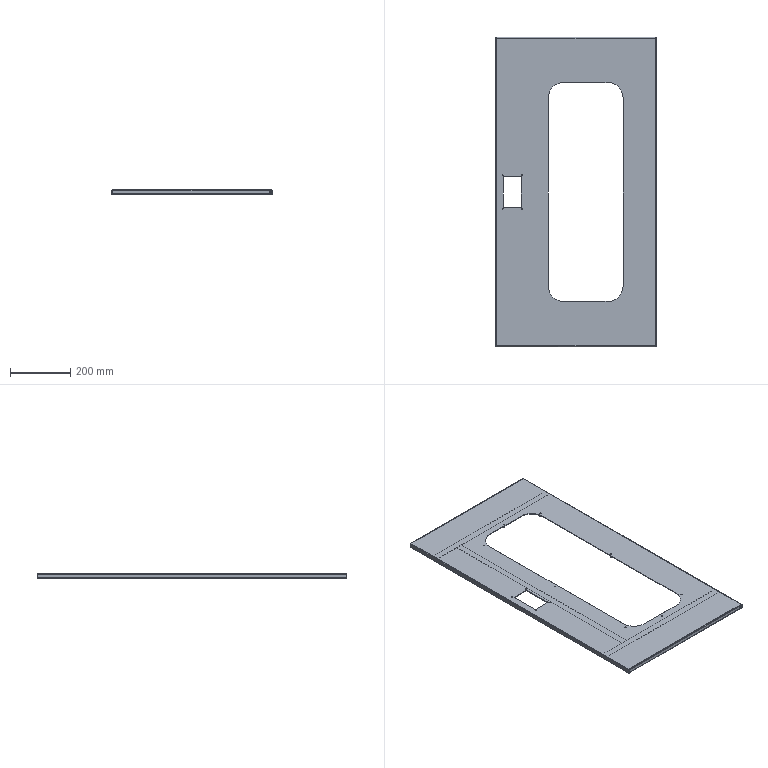Part | STEP file | 4 solids | 238 faces | box 533 x 1028 x 15 mm | volume 886970 mm3 | plane 142 | cylinder 84 | spline 12 | commonest cylinder face diameters 5 x40 1 x14 3.3 x8 4.6 x8 3.4 x6 7 x4